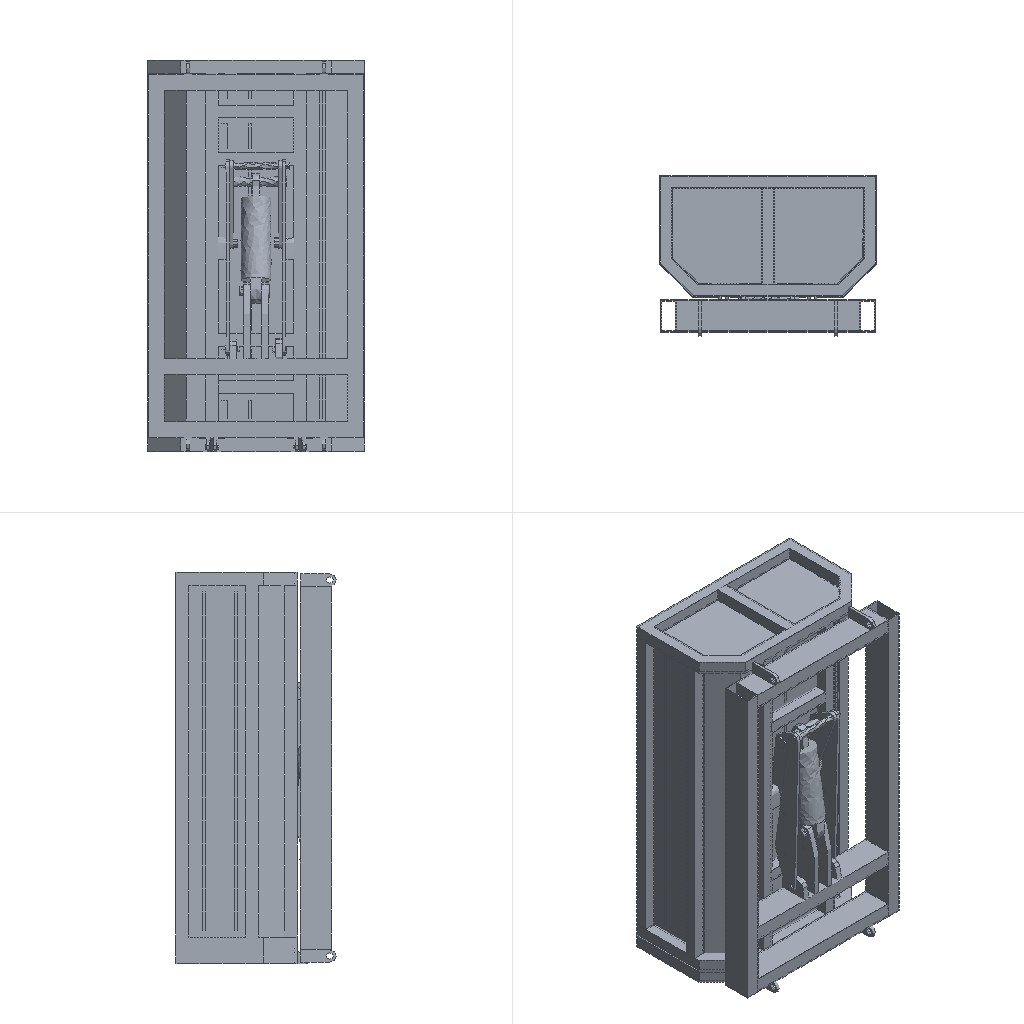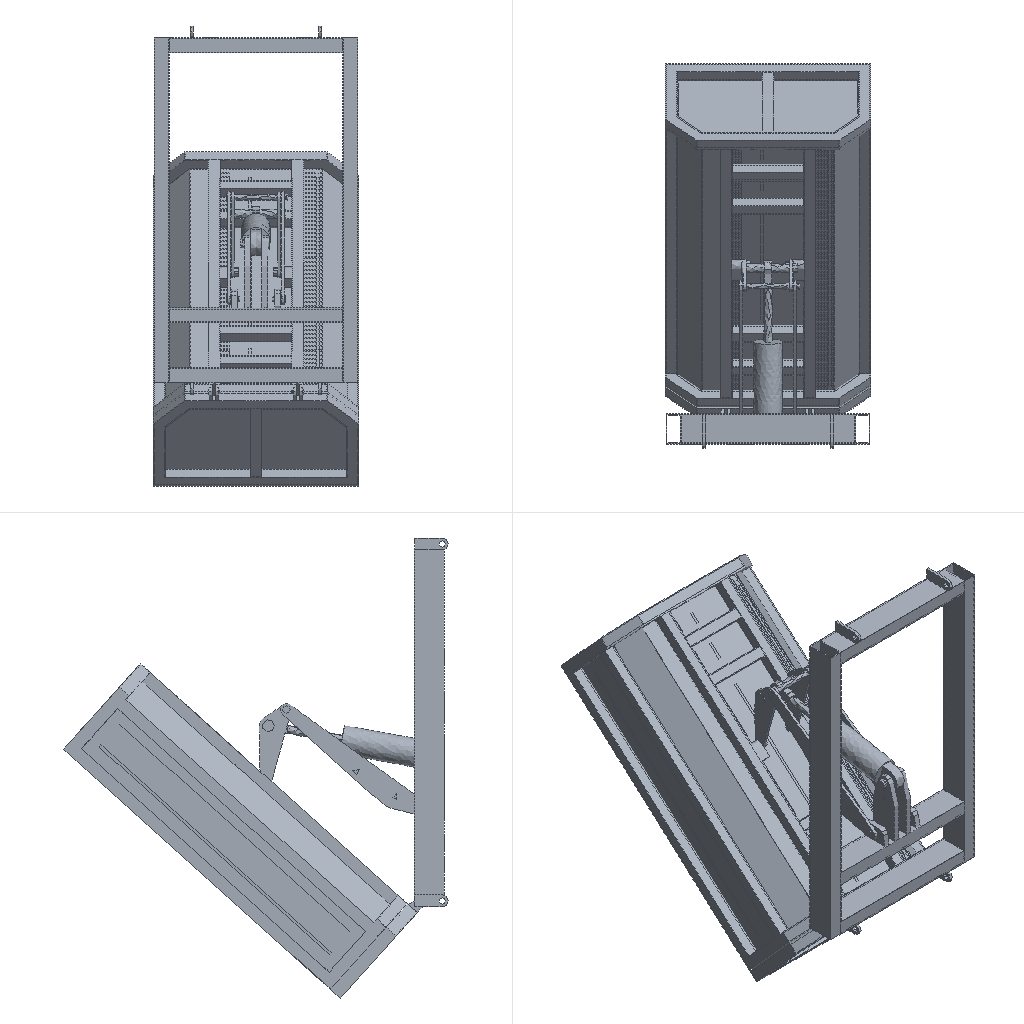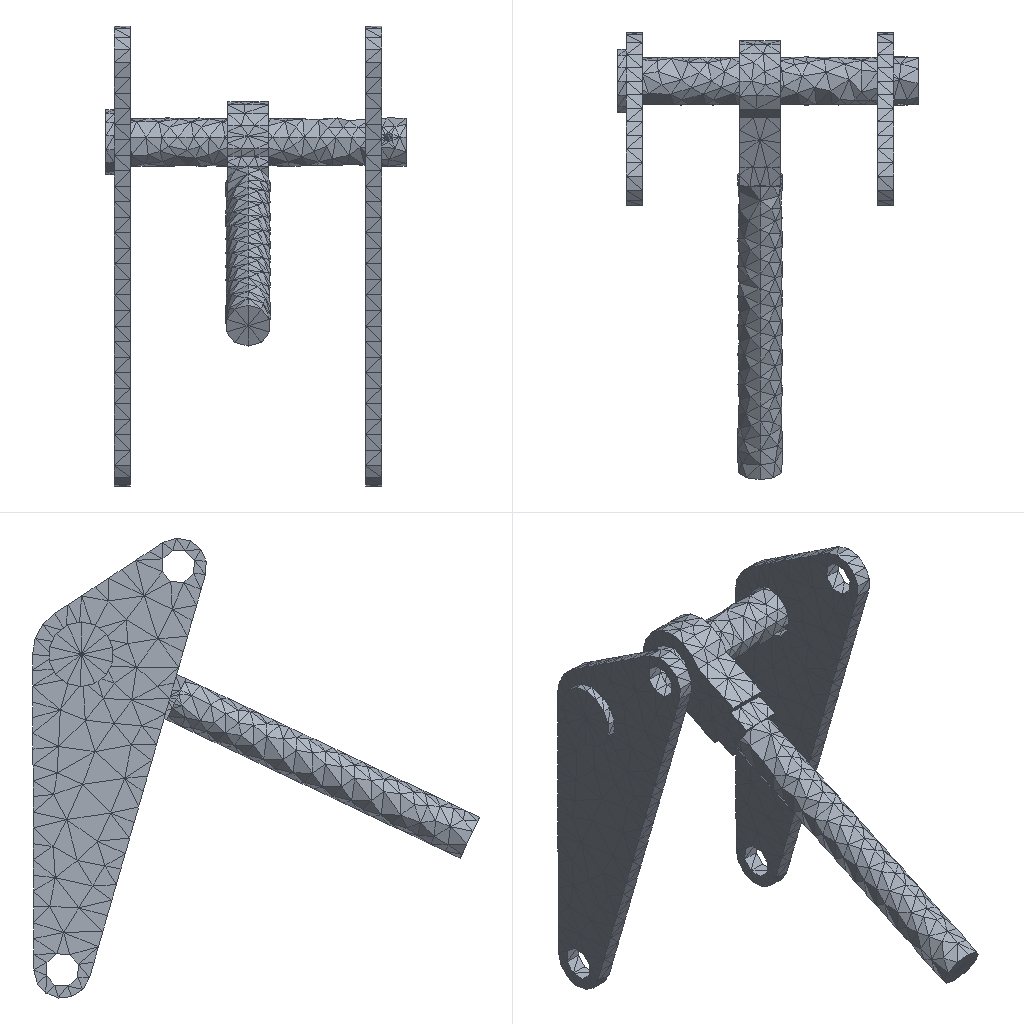Simulation study | ansys workbench
Set-up summary:
category,name,step,type,value,unit,region
solver,ansys_workbench
units,mm-N-s-tonne (MPa),,stated,"/units,MPA"
analysis,deck-1/LS1,,static
load_step,deck-1/LS1,deck-1/LS1,static,nsubst=1; time=1
analysis,deck-2/LS1,,static
load_step,deck-2/LS1,deck-2/LS1,static,nsubst=1; time=1
analysis,deck-3/LS1,,static
load_step,deck-3/LS1,deck-3/LS1,static,nsubst=5; time=1
mesh,deck-1.dat,,nodes,236995
mesh,deck-1.dat,,elements,124539
element_type,SOLID187,,,88763,,deck-1.dat
element_type,CONTA174,,,16770,,deck-1.dat
element_type,TARGE170,,,9810,,deck-1.dat
element_type,SOLID186,,,9154,,deck-1.dat
element_type,SURF154,,,42,,deck-1.dat
mesh,deck-2.dat,,nodes,239345
mesh,deck-2.dat,,elements,125462
element_type,SOLID187,,,92093,,deck-2.dat
element_type,CONTA174,,,14593,,deck-2.dat
element_type,TARGE170,,,10138,,deck-2.dat
element_type,SOLID186,,,8638,,deck-2.dat
mesh,deck-3.dat,,nodes,6791
mesh,deck-3.dat,,elements,4407
element_type,SOLID187,,,3155,,deck-3.dat
element_type,TARGE170,,,596,,deck-3.dat
element_type,CONTA174,,,596,,deck-3.dat
element_type,SURF154,,,60,,deck-3.dat
material,Structural Steel,,E,2e+11,Pa
material,Structural Steel,,nu,0.3
material,Structural Steel,,density,7850,kg m^-3
material,Structural Steel,,conductivity,60.5,W m^-1 C^-1
material,Structural Steel,,specific_heat,434,J kg^-1 C^-1
material,Structural Steel,,cte,1.2e-05,C^-1
material,Structural Steel,,permeability,10000
material,Structural Steel,,resistivity,1.7e-07,kg m^3 A^-2 s^-3
material,Structural Steel,,E,200000,tonne s^-2 mm^-1
material,Structural Steel,,nu,0.3
material,Structural Steel,,density,7.85e-09,tonne mm^-3
material,Structural Steel,,conductivity,60.5,tonne mm s^-3 C^-1
material,Structural Steel,,specific_heat,4.34e+08,mm^2 s^-2 C^-1
material,Structural Steel,,cte,1.2e-05,C^-1
material,Structural Steel,,permeability,10000
material,Structural Steel,,resistivity,0.00017,ohm mm
material,Structural Steel,,E,200000,tonne s^-2 mm^-1
material,Structural Steel,,nu,0.3
material,Structural Steel,,density,7.85e-09,tonne mm^-3
material,Structural Steel,,conductivity,60.5,tonne mm s^-3 C^-1
material,Structural Steel,,specific_heat,4.34e+08,mm^2 s^-2 C^-1
material,Structural Steel,,cte,1.2e-05,C^-1
material,Structural Steel,,permeability,10000
material,Structural Steel,,resistivity,0.00017,ohm mm
load,Define Force Using Surface Effect Elements,deck-1/LS1,surface-effect pres face 2,1.62076e+06,,SURF154 #136
load,Define Force Using Surface Effect Elements,deck-1/LS1,surface-effect pres face 3,1.04112e+07,,SURF154 #136
load,Define Force Using Surface Effect Elements,deck-1/LS1,surface-effect pres face 1,6.74034e-09,,SURF154 #137
load,Define Force Using Surface Effect Elements,deck-1/LS1,surface-effect pres face 2,-1.0493e+06,,SURF154 #137
load,Define Force Using Surface Effect Elements,deck-1/LS1,surface-effect pres face 3,-6.74034e+06,,SURF154 #137
load,ACEL,deck-1/LS1,gravity (ACEL; gravity acts opposite),"9.807 [dir=(0, -1, 0)]",,all
load,ACEL,deck-2/LS1,gravity (ACEL; gravity acts opposite),"9806.65 [dir=(0, -1, 0)]",,all
load,Define Force Using Surface Effect Elements,deck-3/LS1,surface-effect pres face 2,9.527,,SURF154 #9
load,Define Force Using Surface Effect Elements,deck-3/LS1,surface-effect pres face 3,4.496,,SURF154 #9
bc,Fixed Supports,deck-1/model,fixed,[dofs=ALL],,_FIXEDSU
bc,Fixed Supports,deck-2/model,fixed,[dofs=ALL],,_FIXEDSU
bc,Fixed Supports,deck-3/model,fixed,[dofs=ALL],,_FIXEDSU
contact,Contact Region,,bonded (always),element=CONTA174
contact,Contact Region 2,,bonded (always),element=CONTA174
contact,Contact Region 3,,bonded (always),element=CONTA174
contact,Contact Region 8,,bonded (always),element=CONTA174
contact,Contact Region 9,,bonded (always),element=CONTA174
contact,Contact Region 10,,bonded (always),element=CONTA174
contact,Contact Region 13,,bonded (always),element=CONTA174
contact,Contact Region 14,,bonded (always),element=CONTA174
contact,Contact Region 15,,bonded (always),element=CONTA174
contact,Contact Region 16,,bonded (always),element=CONTA174
contact,Contact Region 17,,bonded (always),element=CONTA174
contact,Contact Region 20,,bonded (always),element=CONTA174
contact,Contact Region 21,,bonded (always),element=CONTA174
contact,Contact Region 24,,bonded (always),element=CONTA174
contact,Contact Region 25,,bonded (always),element=CONTA174
contact,Contact Region 26,,bonded (always),element=CONTA174
contact,Contact Region 27,,bonded (always),element=CONTA174
contact,Contact Region 28,,bonded (always),element=CONTA174
contact,Contact Region 29,,bonded (always),element=CONTA174
contact,Contact Region 32,,bonded (always),element=CONTA174
contact,Contact Region 33,,bonded (always),element=CONTA174
contact,Contact Region 36,,bonded (always),element=CONTA174
contact,Contact Region 37,,bonded (always),element=CONTA174
contact,Contact Region 38,,bonded (always),element=CONTA174
contact,Contact Region 39,,bonded (always),element=CONTA174
contact,Contact Region 41,,bonded (always),element=CONTA174
contact,Contact Region 42,,bonded (always),element=CONTA174
contact,Contact Region 44,,bonded (always),element=CONTA174
contact,Contact Region 45,,bonded (always),element=CONTA174
contact,Contact Region 46,,bonded (always),element=CONTA174
contact,Contact Region 47,,bonded (always),element=CONTA174
contact,Contact Region 48,,bonded (always),element=CONTA174
contact,Contact Region 49,,bonded (always),element=CONTA174
contact,Contact Region 50,,bonded (always),element=CONTA174
contact,Contact Region 51,,bonded (always),element=CONTA174
contact,Contact Region 54,,bonded (always),element=CONTA174
contact,Contact Region 55,,bonded (always),element=CONTA174
contact,Contact Region 56,,bonded (always),element=CONTA174
contact,Contact Region 57,,bonded (always),element=CONTA174
contact,Contact Region 58,,bonded (always),element=CONTA174
contact,Contact Region 59,,bonded (always),element=CONTA174
contact,Contact Region 60,,bonded (always),element=CONTA174
contact,Contact Region 61,,bonded (always),element=CONTA174
contact,Contact Region 62,,bonded (always),element=CONTA174
contact,Contact Region 63,,bonded (always),element=CONTA174
contact,Contact Region 64,,bonded (always),element=CONTA174
contact,Contact Region 65,,bonded (always),element=CONTA174
contact,Contact Region 66,,bonded (always),element=CONTA174
contact,contact 49,,bonded (always),element=CONTA174
contact,Contact Region,,bonded (always),element=CONTA174
contact,Contact Region 8,,bonded (always),element=CONTA174
contact,Contact Region 11,,bonded (always),element=CONTA174
contact,Contact Region 12,,bonded (always),element=CONTA174
contact,Contact Region 15,,bonded (always),element=CONTA174
contact,Contact Region 16,,bonded (always),element=CONTA174
contact,Contact Region 19,,bonded (always),element=CONTA174
contact,Contact Region 20,,bonded (always),element=CONTA174
contact,Contact Region 23,,bonded (always),element=CONTA174
contact,Contact Region 24,,bonded (always),element=CONTA174
contact,Contact Region 26,,bonded (always),element=CONTA174
contact,Contact Region 27,,bonded (always),element=CONTA174
contact,Contact Region 29,,bonded (always),element=CONTA174
contact,Contact Region 30,,bonded (always),element=CONTA174
contact,Contact Region 31,,bonded (always),element=CONTA174
contact,Contact Region 32,,bonded (always),element=CONTA174
contact,Contact Region 33,,bonded (always),element=CONTA174
contact,Contact Region 34,,bonded (always),element=CONTA174
contact,Contact Region 35,,bonded (always),element=CONTA174
contact,Contact Region 36,,bonded (always),element=CONTA174
contact,Contact Region 37,,bonded (always),element=CONTA174
contact,Contact Region 38,,bonded (always),element=CONTA174
contact,Contact Region 39,,bonded (always),element=CONTA174
contact,Contact Region 40,,bonded (always),element=CONTA174
contact,Contact Region 41,,bonded (always),element=CONTA174
contact,Contact Region 42,,bonded (always),element=CONTA174
contact,Contact Region 43,,bonded (always),element=CONTA174
contact,Contact Region 44,,bonded (always),element=CONTA174
contact,Contact Region 45,,bonded (always),element=CONTA174
contact,Contact Region 46,,bonded (always),element=CONTA174
contact,contact 31,,bonded (always),element=CONTA174
contact,Frictional - ?28?250|____-____2 ? M30X180?|____-____1,,standard (frictionless/frictional),friction=0.3; element=CONTA174
contact,Bonded - M30X180?|____-____1 ? ?,,bonded (always),element=CONTA174
named_set,_FIXEDSU,,node,160
named_set,_FIXEDSU,,node,348
named_set,_FIXEDSU,,node,108
Results summary:
result,analyses[0].index,,,1
result,analyses[0].system,,,SYS
result,analyses[0].deck,,,deck-1.dat
result,analyses[0].solve_status,,,completed
result,analyses[0].analysis_type,,,static
result,analyses[0].physics,,,mechanical
result,analyses[0].unit_system,,,"MKS: m, kg, N, s, V, A, degC"
result,analyses[0].n_sets,,,1
result,analyses[0].load_steps[0].set,set=1,,1
result,analyses[0].load_steps[0].time_or_freq,set=1,,1
result,analyses[0].load_steps[0].max_displacement_magnitude,set=1,,7.28118e-05
result,analyses[0].load_steps[0].max_von_mises_nodal,set=1,,1.25977e+08
result,analyses[0].load_steps[0].reaction_force_sum_xyz[1],set=1,,1.40995e-05
result,analyses[0].load_steps[0].reaction_force_sum_xyz[2],set=1,,7439.43
result,analyses[0].load_steps[0].reaction_force_sum_xyz[3],set=1,,3.487
result,analyses[1].index,,,2
result,analyses[1].system,,,SYS-1
result,analyses[1].deck,,,deck-2.dat
result,analyses[1].solve_status,,,completed
result,analyses[1].analysis_type,,,static
result,analyses[1].physics,,,mechanical
result,analyses[1].unit_system,,,"NMM: mm, ton, N, s, mV, mA, degC"
result,analyses[1].n_sets,,,1
result,analyses[1].load_steps[0].set,set=1,,1
result,analyses[1].load_steps[0].time_or_freq,set=1,,1
result,analyses[1].load_steps[0].max_displacement_magnitude,set=1,,0.0557
result,analyses[1].load_steps[0].max_von_mises_nodal,set=1,,78.707
result,analyses[1].load_steps[0].reaction_force_sum_xyz[1],set=1,,-3.31264e-05
result,analyses[1].load_steps[0].reaction_force_sum_xyz[2],set=1,,6457.62
result,analyses[1].load_steps[0].reaction_force_sum_xyz[3],set=1,,-1.55365e-05
result,analyses[2].index,,,3
result,analyses[2].system,,,SYS-2
result,analyses[2].deck,,,deck-3.dat
result,analyses[2].solve_status,,,completed
result,analyses[2].analysis_type,,,static
result,analyses[2].physics,,,mechanical
result,analyses[2].unit_system,,,"NMM: mm, ton, N, s, mV, mA, degC"
result,analyses[2].n_sets,,,4
result,analyses[2].load_steps[0].set,set=4,,4
result,analyses[2].load_steps[0].time_or_freq,set=4,,1
result,analyses[2].load_steps[0].max_displacement_magnitude,set=4,,0.2846
result,analyses[2].load_steps[0].max_von_mises_nodal,set=4,,325.541
result,analyses[2].load_steps[0].reaction_force_sum_xyz[1],set=4,,-2.92403e-10
result,analyses[2].load_steps[0].reaction_force_sum_xyz[2],set=4,,-27130.6
result,analyses[2].load_steps[0].reaction_force_sum_xyz[3],set=4,,-12802.9
result,geometry_export[0][0],,,1.step
result,geometry_export[0][1],,,ok
result,geometry_export[0][2],,,39
result,geometry_export[1][0],,,2.step
result,geometry_export[1][1],,,ok
result,geometry_export[1][2],,,24